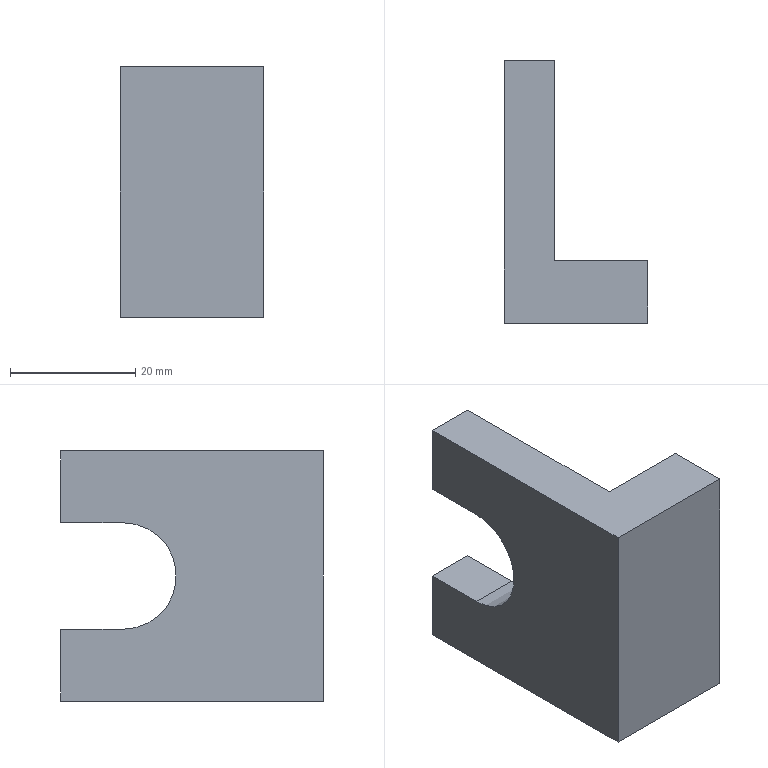Part | SolidWorks | features Extrusion 1, ICE 1 | 1 solid | 12 faces | box 23 x 42 x 40 mm | volume 17172 mm3 | plane 11 | cylinder 1 | commonest cylinder face diameters 17 x1
STEP:
#1=CARTESIAN_POINT('',(0.,42.,-8.5));
#2=VERTEX_POINT('',#1);
#3=CARTESIAN_POINT('',(0.,42.,-20.));
#4=VERTEX_POINT('',#3);
#5=CARTESIAN_POINT('',(0.,42.,20.));
#6=DIRECTION('',(0.,0.,-1.));
#7=VECTOR('',#6,1000.);
#8=LINE('',#5,#7);
#9=EDGE_CURVE('',#2,#4,#8,.T.);
#10=ORIENTED_EDGE('',*,*,#9,.F.);
#11=CARTESIAN_POINT('',(8.,42.,-8.5));
#12=VERTEX_POINT('',#11);
#13=CARTESIAN_POINT('',(-0.001,42.,-8.5));
#14=DIRECTION('',(1.,0.,0.));
#15=VECTOR('',#14,1000.);
#16=LINE('',#13,#15);
#17=EDGE_CURVE('',#2,#12,#16,.T.);
#18=ORIENTED_EDGE('',*,*,#17,.T.);
#19=CARTESIAN_POINT('',(8.,42.,-20.));
#20=VERTEX_POINT('',#19);
#21=CARTESIAN_POINT('',(8.,42.,20.));
#22=DIRECTION('',(0.,0.,-1.));
#23=VECTOR('',#22,1000.);
#24=LINE('',#21,#23);
#25=EDGE_CURVE('',#12,#20,#24,.T.);
#26=ORIENTED_EDGE('',*,*,#25,.T.);
#27=CARTESIAN_POINT('',(8.,42.,-20.));
#28=DIRECTION('',(-1.,0.,0.));
#29=VECTOR('',#28,1000.);
#30=LINE('',#27,#29);
#31=EDGE_CURVE('',#20,#4,#30,.T.);
#32=ORIENTED_EDGE('',*,*,#31,.T.);
#33=EDGE_LOOP('',(#10,#18,#26,#32));
#34=FACE_OUTER_BOUND('',#33,.T.);
#35=CARTESIAN_POINT('',(8.,42.,20.));
#36=DIRECTION('',(0.,-1.,0.));
#37=DIRECTION('',(0.,0.,-1.));
#38=AXIS2_PLACEMENT_3D('',#35,#36,#37);
#39=PLANE('',#38);
#40=ADVANCED_FACE('',(#34),#39,.F.);
#41=CARTESIAN_POINT('',(0.,32.,-8.5));
#42=VERTEX_POINT('',#41);
#43=CARTESIAN_POINT('',(0.,32.,8.5));
#44=VERTEX_POINT('',#43);
#45=CARTESIAN_POINT('',(0.,32.,0.));
#46=DIRECTION('',(-1.,0.,0.));
#47=DIRECTION('',(0.,1.,0.));
#48=AXIS2_PLACEMENT_3D('',#45,#46,#47);
#49=CIRCLE('',#48,8.5);
#50=EDGE_CURVE('',#42,#44,#49,.T.);
#51=ORIENTED_EDGE('',*,*,#50,.F.);
#52=CARTESIAN_POINT('',(0.,32.,-8.5));
#53=DIRECTION('',(0.,-1.,0.));
#54=VECTOR('',#53,1000.);
#55=LINE('',#52,#54);
#56=EDGE_CURVE('',#2,#42,#55,.T.);
#57=ORIENTED_EDGE('',*,*,#56,.F.);
#58=ORIENTED_EDGE('',*,*,#9,.T.);
#59=CARTESIAN_POINT('',(0.,0.,-20.));
#60=VERTEX_POINT('',#59);
#61=CARTESIAN_POINT('',(0.,42.,-20.));
#62=DIRECTION('',(0.,-1.,0.));
#63=VECTOR('',#62,1000.);
#64=LINE('',#61,#63);
#65=EDGE_CURVE('',#4,#60,#64,.T.);
#66=ORIENTED_EDGE('',*,*,#65,.T.);
#67=CARTESIAN_POINT('',(0.,0.,20.));
#68=VERTEX_POINT('',#67);
#69=CARTESIAN_POINT('',(0.,0.,20.));
#70=DIRECTION('',(0.,0.,-1.));
#71=VECTOR('',#70,1000.);
#72=LINE('',#69,#71);
#73=EDGE_CURVE('',#68,#60,#72,.T.);
#74=ORIENTED_EDGE('',*,*,#73,.F.);
#75=CARTESIAN_POINT('',(0.,42.,20.));
#76=VERTEX_POINT('',#75);
#77=CARTESIAN_POINT('',(0.,42.,20.));
#78=DIRECTION('',(0.,-1.,0.));
#79=VECTOR('',#78,1000.);
#80=LINE('',#77,#79);
#81=EDGE_CURVE('',#76,#68,#80,.T.);
#82=ORIENTED_EDGE('',*,*,#81,.F.);
#83=CARTESIAN_POINT('',(0.,42.,8.5));
#84=VERTEX_POINT('',#83);
#85=CARTESIAN_POINT('',(0.,42.,20.));
#86=DIRECTION('',(0.,0.,-1.));
#87=VECTOR('',#86,1000.);
#88=LINE('',#85,#87);
#89=EDGE_CURVE('',#76,#84,#88,.T.);
#90=ORIENTED_EDGE('',*,*,#89,.T.);
#91=CARTESIAN_POINT('',(0.,42.,8.5));
#92=DIRECTION('',(0.,1.,0.));
#93=VECTOR('',#92,1000.);
#94=LINE('',#91,#93);
#95=EDGE_CURVE('',#44,#84,#94,.T.);
#96=ORIENTED_EDGE('',*,*,#95,.F.);
#97=EDGE_LOOP('',(#51,#57,#58,#66,#74,#82,#90,#96));
#98=FACE_OUTER_BOUND('',#97,.T.);
#99=CARTESIAN_POINT('',(0.,42.,20.));
#100=DIRECTION('',(1.,0.,0.));
#101=DIRECTION('',(0.,1.,0.));
#102=AXIS2_PLACEMENT_3D('',#99,#100,#101);
#103=PLANE('',#102);
#104=ADVANCED_FACE('',(#98),#103,.F.);
#105=CARTESIAN_POINT('',(23.,0.,-20.));
#106=VERTEX_POINT('',#105);
#107=CARTESIAN_POINT('',(0.,0.,-20.));
#108=DIRECTION('',(1.,0.,0.));
#109=VECTOR('',#108,1000.);
#110=LINE('',#107,#109);
#111=EDGE_CURVE('',#60,#106,#110,.T.);
#112=ORIENTED_EDGE('',*,*,#111,.T.);
#113=CARTESIAN_POINT('',(23.,0.,20.));
#114=VERTEX_POINT('',#113);
#115=CARTESIAN_POINT('',(23.,0.,20.));
#116=DIRECTION('',(0.,0.,-1.));
#117=VECTOR('',#116,1000.);
#118=LINE('',#115,#117);
#119=EDGE_CURVE('',#114,#106,#118,.T.);
#120=ORIENTED_EDGE('',*,*,#119,.F.);
#121=CARTESIAN_POINT('',(0.,0.,20.));
#122=DIRECTION('',(1.,0.,0.));
#123=VECTOR('',#122,1000.);
#124=LINE('',#121,#123);
#125=EDGE_CURVE('',#68,#114,#124,.T.);
#126=ORIENTED_EDGE('',*,*,#125,.F.);
#127=ORIENTED_EDGE('',*,*,#73,.T.);
#128=EDGE_LOOP('',(#112,#120,#126,#127));
#129=FACE_OUTER_BOUND('',#128,.T.);
#130=CARTESIAN_POINT('',(0.,0.,20.));
#131=DIRECTION('',(0.,1.,0.));
#132=DIRECTION('',(0.,0.,1.));
#133=AXIS2_PLACEMENT_3D('',#130,#131,#132);
#134=PLANE('',#133);
#135=ADVANCED_FACE('',(#129),#134,.F.);
#136=CARTESIAN_POINT('',(23.,10.,-20.));
#137=VERTEX_POINT('',#136);
#138=CARTESIAN_POINT('',(23.,0.,-20.));
#139=DIRECTION('',(0.,1.,0.));
#140=VECTOR('',#139,1000.);
#141=LINE('',#138,#140);
#142=EDGE_CURVE('',#106,#137,#141,.T.);
#143=ORIENTED_EDGE('',*,*,#142,.T.);
#144=CARTESIAN_POINT('',(23.,10.,20.));
#145=VERTEX_POINT('',#144);
#146=CARTESIAN_POINT('',(23.,10.,20.));
#147=DIRECTION('',(0.,0.,-1.));
#148=VECTOR('',#147,1000.);
#149=LINE('',#146,#148);
#150=EDGE_CURVE('',#145,#137,#149,.T.);
#151=ORIENTED_EDGE('',*,*,#150,.F.);
#152=CARTESIAN_POINT('',(23.,0.,20.));
#153=DIRECTION('',(0.,1.,0.));
#154=VECTOR('',#153,1000.);
#155=LINE('',#152,#154);
#156=EDGE_CURVE('',#114,#145,#155,.T.);
#157=ORIENTED_EDGE('',*,*,#156,.F.);
#158=ORIENTED_EDGE('',*,*,#119,.T.);
#159=EDGE_LOOP('',(#143,#151,#157,#158));
#160=FACE_OUTER_BOUND('',#159,.T.);
#161=CARTESIAN_POINT('',(23.,0.,20.));
#162=DIRECTION('',(-1.,0.,0.));
#163=DIRECTION('',(0.,0.,1.));
#164=AXIS2_PLACEMENT_3D('',#161,#162,#163);
#165=PLANE('',#164);
#166=ADVANCED_FACE('',(#160),#165,.F.);
#167=CARTESIAN_POINT('',(8.,10.,-20.));
#168=VERTEX_POINT('',#167);
#169=CARTESIAN_POINT('',(23.,10.,-20.));
#170=DIRECTION('',(-1.,0.,0.));
#171=VECTOR('',#170,1000.);
#172=LINE('',#169,#171);
#173=EDGE_CURVE('',#137,#168,#172,.T.);
#174=ORIENTED_EDGE('',*,*,#173,.T.);
#175=CARTESIAN_POINT('',(8.,10.,20.));
#176=VERTEX_POINT('',#175);
#177=CARTESIAN_POINT('',(8.,10.,20.));
#178=DIRECTION('',(0.,0.,-1.));
#179=VECTOR('',#178,1000.);
#180=LINE('',#177,#179);
#181=EDGE_CURVE('',#176,#168,#180,.T.);
#182=ORIENTED_EDGE('',*,*,#181,.F.);
#183=CARTESIAN_POINT('',(23.,10.,20.));
#184=DIRECTION('',(-1.,0.,0.));
#185=VECTOR('',#184,1000.);
#186=LINE('',#183,#185);
#187=EDGE_CURVE('',#145,#176,#186,.T.);
#188=ORIENTED_EDGE('',*,*,#187,.F.);
#189=ORIENTED_EDGE('',*,*,#150,.T.);
#190=EDGE_LOOP('',(#174,#182,#188,#189));
#191=FACE_OUTER_BOUND('',#190,.T.);
#192=CARTESIAN_POINT('',(23.,10.,20.));
#193=DIRECTION('',(0.,-1.,0.));
#194=DIRECTION('',(1.,0.,0.));
#195=AXIS2_PLACEMENT_3D('',#192,#193,#194);
#196=PLANE('',#195);
#197=ADVANCED_FACE('',(#191),#196,.F.);
#198=ORIENTED_EDGE('',*,*,#25,.F.);
#199=CARTESIAN_POINT('',(8.,32.,-8.5));
#200=VERTEX_POINT('',#199);
#201=CARTESIAN_POINT('',(8.,32.,-8.5));
#202=DIRECTION('',(0.,1.,0.));
#203=VECTOR('',#202,1000.);
#204=LINE('',#201,#203);
#205=EDGE_CURVE('',#200,#12,#204,.T.);
#206=ORIENTED_EDGE('',*,*,#205,.F.);
#207=CARTESIAN_POINT('',(8.,32.,8.5));
#208=VERTEX_POINT('',#207);
#209=CARTESIAN_POINT('',(8.,32.,0.));
#210=DIRECTION('',(1.,0.,0.));
#211=DIRECTION('',(0.,1.,0.));
#212=AXIS2_PLACEMENT_3D('',#209,#210,#211);
#213=CIRCLE('',#212,8.5);
#214=EDGE_CURVE('',#208,#200,#213,.T.);
#215=ORIENTED_EDGE('',*,*,#214,.F.);
#216=CARTESIAN_POINT('',(8.,42.,8.5));
#217=VERTEX_POINT('',#216);
#218=CARTESIAN_POINT('',(8.,42.,8.5));
#219=DIRECTION('',(0.,-1.,0.));
#220=VECTOR('',#219,1000.);
#221=LINE('',#218,#220);
#222=EDGE_CURVE('',#217,#208,#221,.T.);
#223=ORIENTED_EDGE('',*,*,#222,.F.);
#224=CARTESIAN_POINT('',(8.,42.,20.));
#225=VERTEX_POINT('',#224);
#226=CARTESIAN_POINT('',(8.,42.,20.));
#227=DIRECTION('',(0.,0.,-1.));
#228=VECTOR('',#227,1000.);
#229=LINE('',#226,#228);
#230=EDGE_CURVE('',#225,#217,#229,.T.);
#231=ORIENTED_EDGE('',*,*,#230,.F.);
#232=CARTESIAN_POINT('',(8.,10.,20.));
#233=DIRECTION('',(0.,1.,0.));
#234=VECTOR('',#233,1000.);
#235=LINE('',#232,#234);
#236=EDGE_CURVE('',#176,#225,#235,.T.);
#237=ORIENTED_EDGE('',*,*,#236,.F.);
#238=ORIENTED_EDGE('',*,*,#181,.T.);
#239=CARTESIAN_POINT('',(8.,10.,-20.));
#240=DIRECTION('',(0.,1.,0.));
#241=VECTOR('',#240,1000.);
#242=LINE('',#239,#241);
#243=EDGE_CURVE('',#168,#20,#242,.T.);
#244=ORIENTED_EDGE('',*,*,#243,.T.);
#245=EDGE_LOOP('',(#198,#206,#215,#223,#231,#237,#238,#244));
#246=FACE_OUTER_BOUND('',#245,.T.);
#247=CARTESIAN_POINT('',(8.,10.,20.));
#248=DIRECTION('',(-1.,0.,0.));
#249=DIRECTION('',(0.,-1.,0.));
#250=AXIS2_PLACEMENT_3D('',#247,#248,#249);
#251=PLANE('',#250);
#252=ADVANCED_FACE('',(#246),#251,.F.);
#253=ORIENTED_EDGE('',*,*,#230,.T.);
#254=CARTESIAN_POINT('',(-0.001,42.,8.5));
#255=DIRECTION('',(1.,0.,0.));
#256=VECTOR('',#255,1000.);
#257=LINE('',#254,#256);
#258=EDGE_CURVE('',#84,#217,#257,.T.);
#259=ORIENTED_EDGE('',*,*,#258,.F.);
#260=ORIENTED_EDGE('',*,*,#89,.F.);
#261=CARTESIAN_POINT('',(8.,42.,20.));
#262=DIRECTION('',(-1.,0.,0.));
#263=VECTOR('',#262,1000.);
#264=LINE('',#261,#263);
#265=EDGE_CURVE('',#225,#76,#264,.T.);
#266=ORIENTED_EDGE('',*,*,#265,.F.);
#267=EDGE_LOOP('',(#253,#259,#260,#266));
#268=FACE_OUTER_BOUND('',#267,.T.);
#269=CARTESIAN_POINT('',(8.,42.,20.));
#270=DIRECTION('',(0.,-1.,0.));
#271=DIRECTION('',(0.,0.,-1.));
#272=AXIS2_PLACEMENT_3D('',#269,#270,#271);
#273=PLANE('',#272);
#274=ADVANCED_FACE('',(#268),#273,.F.);
#275=ORIENTED_EDGE('',*,*,#81,.T.);
#276=ORIENTED_EDGE('',*,*,#125,.T.);
#277=ORIENTED_EDGE('',*,*,#156,.T.);
#278=ORIENTED_EDGE('',*,*,#187,.T.);
#279=ORIENTED_EDGE('',*,*,#236,.T.);
#280=ORIENTED_EDGE('',*,*,#265,.T.);
#281=EDGE_LOOP('',(#275,#276,#277,#278,#279,#280));
#282=FACE_OUTER_BOUND('',#281,.T.);
#283=CARTESIAN_POINT('',(0.,0.,20.));
#284=DIRECTION('',(0.,0.,1.));
#285=DIRECTION('',(1.,0.,0.));
#286=AXIS2_PLACEMENT_3D('',#283,#284,#285);
#287=PLANE('',#286);
#288=ADVANCED_FACE('',(#282),#287,.T.);
#289=ORIENTED_EDGE('',*,*,#65,.F.);
#290=ORIENTED_EDGE('',*,*,#31,.F.);
#291=ORIENTED_EDGE('',*,*,#243,.F.);
#292=ORIENTED_EDGE('',*,*,#173,.F.);
#293=ORIENTED_EDGE('',*,*,#142,.F.);
#294=ORIENTED_EDGE('',*,*,#111,.F.);
#295=EDGE_LOOP('',(#289,#290,#291,#292,#293,#294));
#296=FACE_OUTER_BOUND('',#295,.T.);
#297=CARTESIAN_POINT('',(0.,0.,-20.));
#298=DIRECTION('',(0.,0.,1.));
#299=DIRECTION('',(1.,0.,0.));
#300=AXIS2_PLACEMENT_3D('',#297,#298,#299);
#301=PLANE('',#300);
#302=ADVANCED_FACE('',(#296),#301,.F.);
#303=ORIENTED_EDGE('',*,*,#56,.T.);
#304=CARTESIAN_POINT('',(-0.001,32.,-8.5));
#305=DIRECTION('',(1.,0.,0.));
#306=VECTOR('',#305,1000.);
#307=LINE('',#304,#306);
#308=EDGE_CURVE('',#42,#200,#307,.T.);
#309=ORIENTED_EDGE('',*,*,#308,.T.);
#310=ORIENTED_EDGE('',*,*,#205,.T.);
#311=ORIENTED_EDGE('',*,*,#17,.F.);
#312=EDGE_LOOP('',(#303,#309,#310,#311));
#313=FACE_OUTER_BOUND('',#312,.T.);
#314=CARTESIAN_POINT('',(-0.001,32.,-8.5));
#315=DIRECTION('',(0.,0.,-1.));
#316=DIRECTION('',(-1.,0.,0.));
#317=AXIS2_PLACEMENT_3D('',#314,#315,#316);
#318=PLANE('',#317);
#319=ADVANCED_FACE('',(#313),#318,.F.);
#320=ORIENTED_EDGE('',*,*,#50,.T.);
#321=CARTESIAN_POINT('',(-0.001,32.,8.5));
#322=DIRECTION('',(1.,0.,0.));
#323=VECTOR('',#322,1000.);
#324=LINE('',#321,#323);
#325=EDGE_CURVE('',#44,#208,#324,.T.);
#326=ORIENTED_EDGE('',*,*,#325,.T.);
#327=ORIENTED_EDGE('',*,*,#214,.T.);
#328=ORIENTED_EDGE('',*,*,#308,.F.);
#329=EDGE_LOOP('',(#320,#326,#327,#328));
#330=FACE_OUTER_BOUND('',#329,.T.);
#331=CARTESIAN_POINT('',(-0.001,32.,0.));
#332=DIRECTION('',(1.,0.,0.));
#333=DIRECTION('',(0.,1.,0.));
#334=AXIS2_PLACEMENT_3D('',#331,#332,#333);
#335=CYLINDRICAL_SURFACE('',#334,8.5);
#336=ADVANCED_FACE('',(#330),#335,.F.);
#337=ORIENTED_EDGE('',*,*,#95,.T.);
#338=ORIENTED_EDGE('',*,*,#258,.T.);
#339=ORIENTED_EDGE('',*,*,#222,.T.);
#340=ORIENTED_EDGE('',*,*,#325,.F.);
#341=EDGE_LOOP('',(#337,#338,#339,#340));
#342=FACE_OUTER_BOUND('',#341,.T.);
#343=CARTESIAN_POINT('',(-0.001,42.,8.5));
#344=DIRECTION('',(0.,0.,1.));
#345=DIRECTION('',(0.,-1.,0.));
#346=AXIS2_PLACEMENT_3D('',#343,#344,#345);
#347=PLANE('',#346);
#348=ADVANCED_FACE('',(#342),#347,.F.);
#349=CLOSED_SHELL('',(#40,#104,#135,#166,#197,#252,#274,#288,#302,#319,#336,#348));
#350=MANIFOLD_SOLID_BREP('',#349);
#351=CARTESIAN_POINT('',(0.,0.,0.));
#352=DIRECTION('',(0.,0.,1.));
#353=DIRECTION('',(1.,0.,0.));
#354=AXIS2_PLACEMENT_3D('',#351,#352,#353);
#355=(LENGTH_UNIT()NAMED_UNIT(*)SI_UNIT(.MILLI.,.METRE.));
#356=UNCERTAINTY_MEASURE_WITH_UNIT(LENGTH_MEASURE(0.00001),#355,'','');
#357=(NAMED_UNIT(*)PLANE_ANGLE_UNIT()SI_UNIT($,.RADIAN.));
#358=(NAMED_UNIT(*)SI_UNIT($,.STERADIAN.)SOLID_ANGLE_UNIT());
#359=(GEOMETRIC_REPRESENTATION_CONTEXT(3)GLOBAL_UNCERTAINTY_ASSIGNED_CONTEXT((#356))GLOBAL_UNIT_ASSIGNED_CONTEXT((#355,#357,#358))REPRESENTATION_CONTEXT('',''));
#360=ADVANCED_BREP_SHAPE_REPRESENTATION('',(#350,#354),#359);